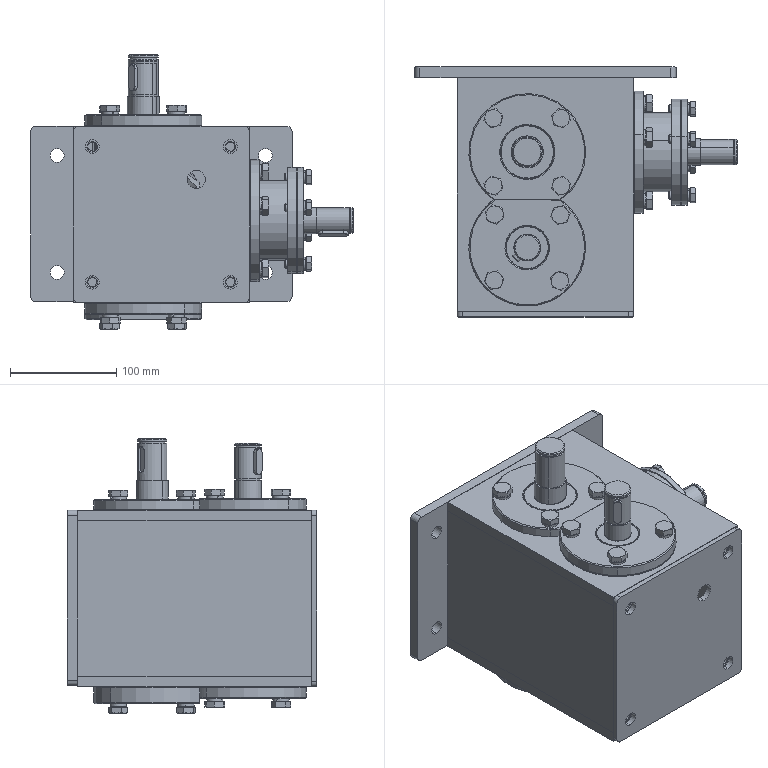Part | SolidWorks | features LayoutProfileFeature 1 | 99 solids | 2713 faces | box 303.75 x 235 x 258.25 mm | volume 3389145 mm3 | cylinder 956 | cone 813 | plane 774 | spline 170 | commonest cylinder face diameters 60.03 x124 11 x72 82.5 x62 10.2 x60 15.4 x60 96 x60